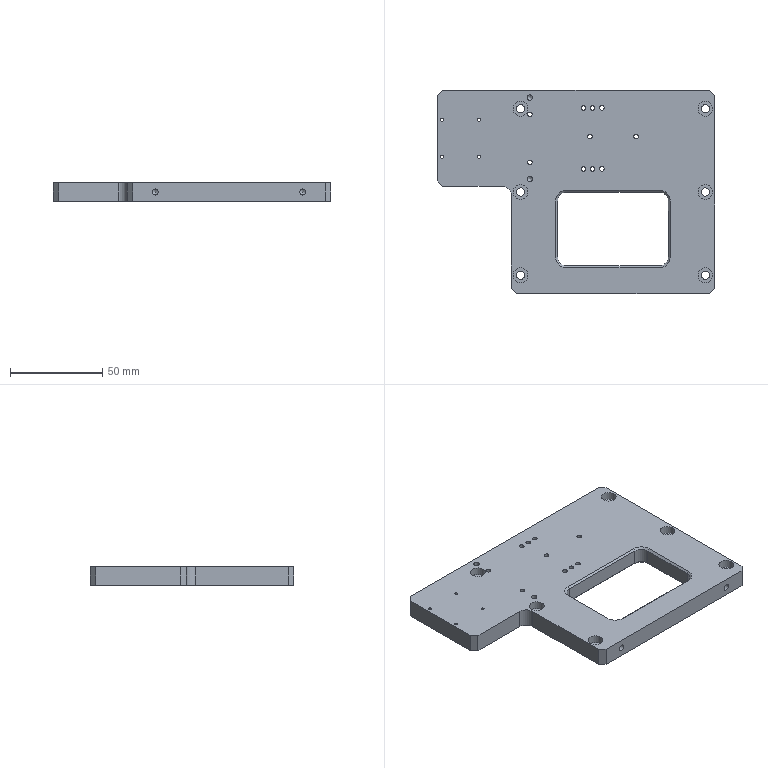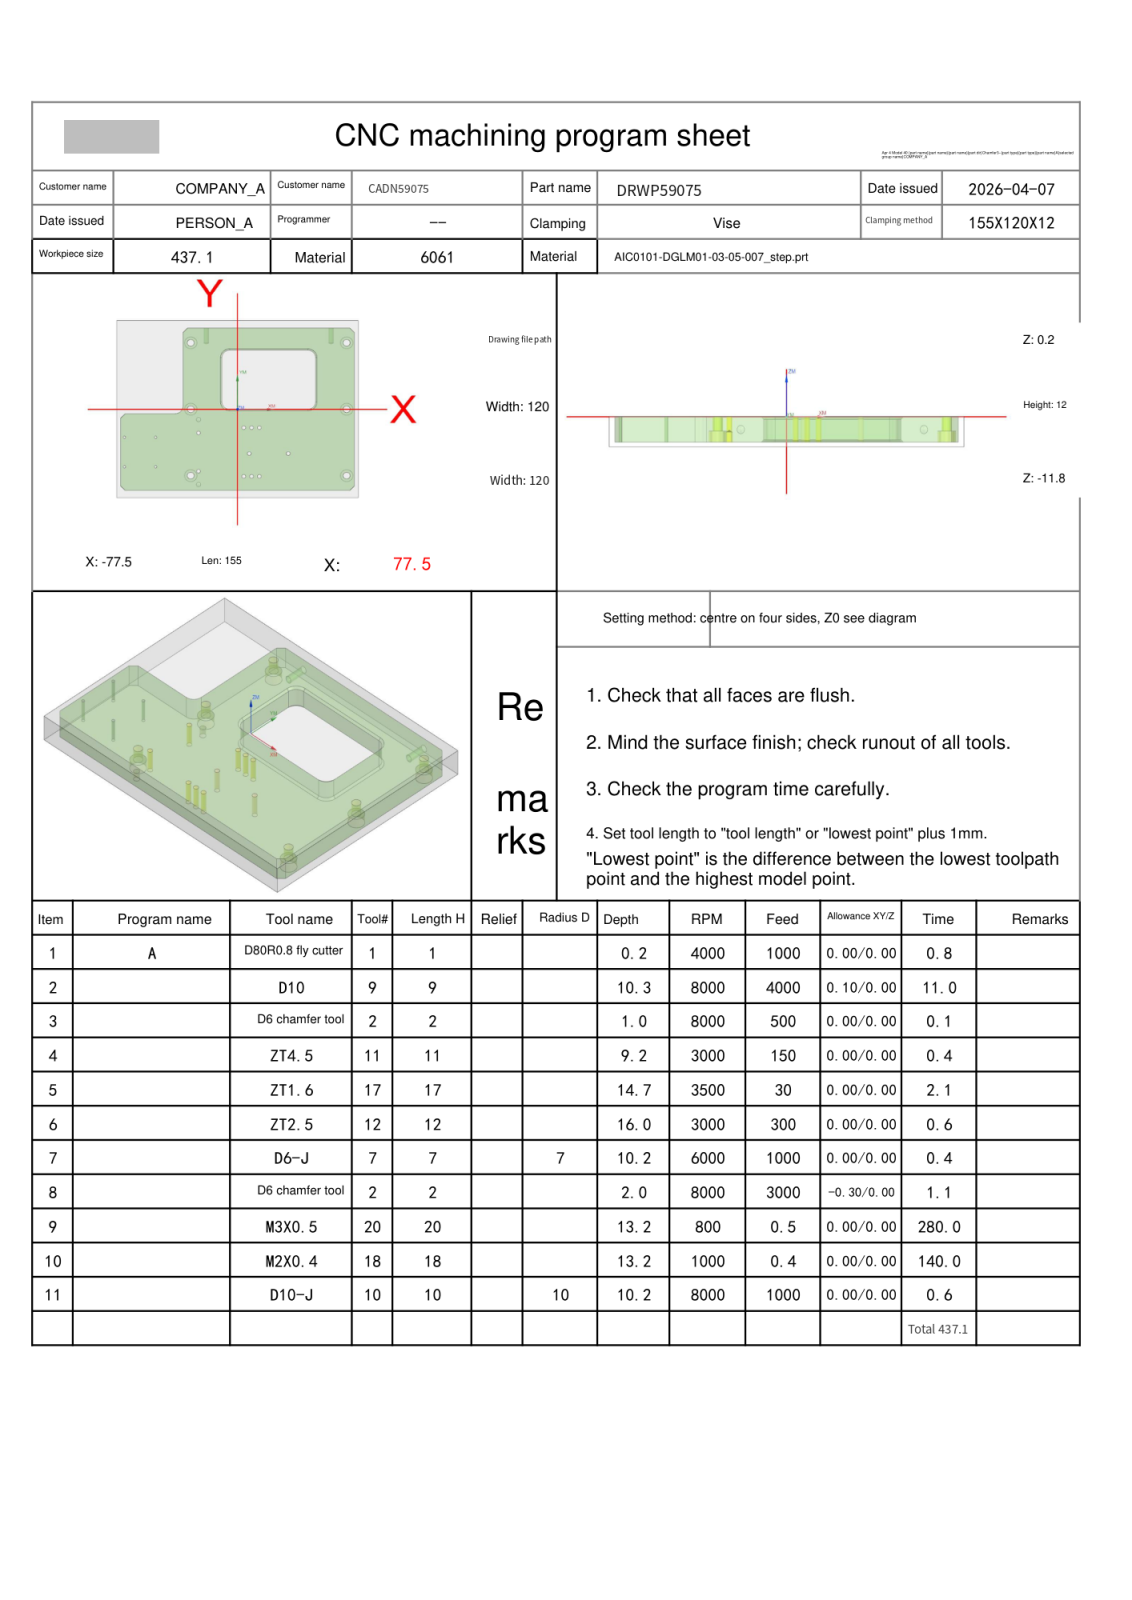NC program | NX | posted by the shop | part box 150 x 110 x 10 mm
Lines 3208 to 3675 of 3675:
N3 T02 M06
(D6 chamfer tool  D=6. R=0. H=02 ce=0.00 di=0.00)
G00 G90 G54 X-30. Y45. M03 S8000
G43 H02 Z20.
M08
G98 G81 X-30. Y45. Z-.8 R1. F500.
Y0.0
X-25. Y-16.
X-52.5 Y-19.
X-72.5
Y-39.
X-52.5
X-30. Y-45.
X-25. Y-42.
X4. Y-45.5
X9.
X14.
X7.5 Y-30.
X4. Y-12.5
X9.
X14.
X32.5 Y-30.
X70. Y-45.
Y0.0
Y45.
G80
G00 Z20.
G91 G28 Z0.0
M05
M09
G91 G28 Z0.0
M01
N4 T11 M06
(ZT4.5 D=4.5 DR_a=118 H=11)
G00 G90 G54 X-30. Y45. M03 S3000
G43 H11 Z20.
M08
G98 G83 X-30. Y45. Z-8.952 R1. F150. Q3.
Y0.0
Y-45.
X70.
Y0.0
Y45.
G80
G00 Z20.
G91 G28 Z0.0
M05
M09
G91 G28 Z0.0
M01
N5 T17 M06
(ZT1.6 D=1.6 DR_a=118 H=17)
G00 G90 G54 X-52.5 Y-39. M03 S3500
G43 H17 Z20.
M08
G98 G83 X-52.5 Y-39. Z-14.481 R1. F30. Q1.
Y-19.
X-72.5
Y-39.
G80
G00 Z20.
G91 G28 Z0.0
M05
M09
G91 G28 Z0.0
M01
N6 T12 M06
(ZT2.5 D=2.5 DR_a=118 H=12)
G00 G90 G54 X32.5 Y-30. M03 S3000
G43 H12 Z20.
M08
G98 G83 X32.5 Y-30. Z-15.751 R1. F300. Q2.
X14. Y-12.5
X9.
X4.
X7.5 Y-30.
X14. Y-45.5
X9.
X4.
X-25. Y-42.
Y-16.
G80
G00 Z20.
G91 G28 Z0.0
M05
M09
G91 G28 Z0.0
M01
N7 T07 M06
(D6-J  D=6. R=0. H=07 ce=0.00 di=0.00)
G00 G90 G54 X46. Y34.8 M03 S6000
G43 H07 Z20.
M08
Z-8.
G01 Z-8.5 F1000.
G41 D07
Y36.
G03 X45. Y37. I-1. J0.0
G01 X-5.
G03 X-7. Y35. I0.0 J-2.
G01 Y5.
G03 X-5. Y3. I2. J0.0
G01 X45.
G03 X47. Y5. I0.0 J2.
G01 Y35.
G03 X45. Y37. I-2. J0.0
G01 X44.5
G03 X43.5 Y36. I0.0 J-1.
G01 G40 Y35.8
Z-8.
G00 Z20.
G00 G90 X46. Y34.9 M03 S6000
Z20.
Z-9.5
G01 Z-10. F1000.
G41 D07
Y36.
G03 X45. Y37. I-1. J0.0
G01 X-5.
G03 X-7. Y35. I0.0 J-2.
G01 Y5.
G03 X-5. Y3. I2. J0.0
G01 X45.
G03 X47. Y5. I0.0 J2.
G01 Y35.
G03 X45. Y37. I-2. J0.0
G01 X44.5
G03 X43.5 Y36. I0.0 J-1.
G01 G40 Y35.9
Z-9.5
G00 Z20.
G91 G28 Z0.0
M05
M09
G91 G28 Z0.0
M01
N8 T02 M06
(D6 chamfer tool  D=6. R=0. H=02 ce=0.00 di=0.00)
G00 G90 G54 X.25 Y-57.128 M03 S8000
G43 H02 Z20.
M08
Z2.099
G01 Z-1.5 F3000.
G03 X.33 Y-56.828 I-.52 J.3
X.03 Y-56.308 I-.6 J0.0
G01 X0.0 Y-56.3
X-72.
X-72.254 Y-56.275
X-72.497 Y-56.201
X-72.722 Y-56.081
X-72.919 Y-55.919
X-75.919 Y-52.919
X-76.081 Y-52.722
X-76.201 Y-52.497
X-76.275 Y-52.254
X-76.3 Y-52.
Y-6.
X-76.275 Y-5.746
X-76.201 Y-5.503
X-76.081 Y-5.278
X-75.919 Y-5.081
X-72.919 Y-2.081
X-72.722 Y-1.919
X-72.497 Y-1.799
X-72.254 Y-1.725
X-72. Y-1.7
X-40.
G03 X-36.3 Y2. I0.0 J3.7
G01 Y52.
X-36.275 Y52.254
X-36.201 Y52.497
X-36.081 Y52.722
X-35.919 Y52.919
X-32.919 Y55.919
X-32.722 Y56.081
X-32.497 Y56.201
X-32.254 Y56.275
X-32. Y56.3
X72.
X72.254 Y56.275
X72.497 Y56.201
X72.722 Y56.081
X72.919 Y55.919
X75.919 Y52.919
X76.081 Y52.722
X76.201 Y52.497
X76.275 Y52.254
X76.3 Y52.
Y-52.
X76.275 Y-52.254
X76.201 Y-52.497
X76.081 Y-52.722
X75.919 Y-52.919
X72.919 Y-55.919
X72.722 Y-56.081
X72.497 Y-56.201
X72.254 Y-56.275
X72. Y-56.3
X0.0
X-.03 Y-56.308
G03 X-.33 Y-56.828 I.3 J-.52
X-.25 Y-57.128 I.6 J0.0
G01 Z2.099
G00 Z20.
G00 G90 X-52.5 Y-39. M03 S8000
Z20.
G98 G81 X-52.5 Y-39. Z-1.2 R3. F500.
Y-19.
X-72.5
Y-39.
G80
G00 Z20.
G00 G90 X32.5 Y-30. M03 S8000
Z20.
G98 G81 X32.5 Y-30. Z-1.75 R3. F500.
X14. Y-12.5
X9.
X4.
X7.5 Y-30.
X14. Y-45.5
X9.
X4.
X-25. Y-42.
Y-16.
G80
G00 Z20.
G00 G90 X69.982 Y45.55 M03 S8000
Z20.
Z-.5
G01 Z-1. F500.
X69.95 Y46.5
G03 X68.45 Y45. I0.0 J-1.5
X70. Y43.45 I1.55 J0.0
X71.55 Y45. I0.0 J1.55
X70. Y46.55 I-1.55 J0.0
X68.45 Y45. I0.0 J-1.55
X69.95 Y43.5 I1.5 J0.0
G01 X69.982 Y44.45
Z-.5
G00 Z20.
Y.55
Z-.5
G01 Z-1.
X69.95 Y1.5
G03 X68.45 Y0.0 I0.0 J-1.5
X70. Y-1.55 I1.55 J0.0
X71.55 Y0.0 I0.0 J1.55
X70. Y1.55 I-1.55 J0.0
X68.45 Y0.0 I0.0 J-1.55
X69.95 Y-1.5 I1.5 J0.0
G01 X69.982 Y-.55
Z-.5
G00 Z20.
Y-44.45
Z-.5
G01 Z-1.
X69.95 Y-43.5
G03 X68.45 Y-45. I0.0 J-1.5
X70. Y-46.55 I1.55 J0.0
X71.55 Y-45. I0.0 J1.55
X70. Y-43.45 I-1.55 J0.0
X68.45 Y-45. I0.0 J-1.55
X69.95 Y-46.5 I1.5 J0.0
G01 X69.982 Y-45.55
Z-.5
G00 Z20.
X-30.018 Y-44.45
Z-.5
G01 Z-1.
X-30.05 Y-43.5
G03 X-31.55 Y-45. I0.0 J-1.5
X-30. Y-46.55 I1.55 J0.0
X-28.45 Y-45. I0.0 J1.55
X-30. Y-43.45 I-1.55 J0.0
X-31.55 Y-45. I0.0 J-1.55
X-30.05 Y-46.5 I1.5 J0.0
G01 X-30.018 Y-45.55
Z-.5
G00 Z20.
Y.55
Z-.5
G01 Z-1.
X-30.05 Y1.5
G03 X-31.55 Y0.0 I0.0 J-1.5
X-30. Y-1.55 I1.55 J0.0
X-28.45 Y0.0 I0.0 J1.55
X-30. Y1.55 I-1.55 J0.0
X-31.55 Y0.0 I0.0 J-1.55
X-30.05 Y-1.5 I1.5 J0.0
G01 X-30.018 Y-.55
Z-.5
G00 Z20.
Y45.55
Z-.5
G01 Z-1.
X-30.05 Y46.5
G03 X-31.55 Y45. I0.0 J-1.5
X-30. Y43.45 I1.55 J0.0
X-28.45 Y45. I0.0 J1.55
X-30. Y46.55 I-1.55 J0.0
X-31.55 Y45. I0.0 J-1.55
X-30.05 Y43.5 I1.5 J0.0
G01 X-30.018 Y44.45
Z-.5
G00 Z20.
G00 G90 X46.2 Y37.193 M03 S6500
Z20.
Z-.2
G01 Z-1.7 F1500.
Y37.5
G03 X45. Y38.7 I-1.2 J0.0
G01 X-5.
G03 X-8.7 Y35. I0.0 J-3.7
G01 Y5.
G03 X-5. Y1.3 I3.7 J0.0
G01 X45.
G03 X48.7 Y5. I0.0 J3.7
G01 Y35.
G03 X48.693 Y35.231 I-3.7 J0.0
G01 X48.681 Y35.372
G03 X48.648 Y35.617 I-3.681 J-.372
X46.911 Y38.169 I-3.648 J-.617
X46.423 Y38.416 I-1.911 J-3.169
X45. Y38.7 I-1.423 J-3.416
G01 X44.6
G03 X43.4 Y37.5 I0.0 J-1.2
G01 X46.2 Y37.7
G03 X45. Y38.9 I-1.2 J0.0
G01 X-5.
G03 X-8.9 Y35. I0.0 J-3.9
G01 Y5.
G03 X-5. Y1.1 I3.9 J0.0
G01 X45.
G03 X48.9 Y5. I0.0 J3.9
G01 Y35.
G03 X48.892 Y35.243 I-3.9 J0.0
G01 X48.88 Y35.392
G03 X48.845 Y35.65 I-3.88 J-.392
X47.014 Y38.34 I-3.845 J-.65
X46.5 Y38.6 I-2.014 J-3.34
X45. Y38.9 I-1.5 J-3.6
G01 X44.6
G03 X43.4 Y37.7 I0.0 J-1.2
G01 X46.2 Y37.9
G03 X45. Y39.1 I-1.2 J0.0
G01 X-5.
G03 X-9.1 Y35. I0.0 J-4.1
G01 Y5.
G03 X-5. Y.9 I4.1 J0.0
G01 X45.
G03 X49.1 Y5. I0.0 J4.1
G01 Y35.
G03 X49.092 Y35.256 I-4.1 J0.0
G01 X49.089 Y35.334
X49.079 Y35.412
G03 X49.043 Y35.684 I-4.079 J-.412
X47.117 Y38.511 I-4.043 J-.684
X46.576 Y38.785 I-2.117 J-3.511
X45. Y39.1 I-1.576 J-3.785
G01 X44.6
G03 X43.4 Y37.9 I0.0 J-1.2
G01 X46.2 Y38.1
G03 X45. Y39.3 I-1.2 J0.0
G01 X-5.
G03 X-9.3 Y35. I0.0 J-4.3
G01 Y5.
G03 X-5. Y.7 I4.3 J0.0
G01 X45.
G03 X49.3 Y5. I0.0 J4.3
G01 Y35.
G03 X49.292 Y35.268 I-4.3 J0.0
G01 X49.289 Y35.351
X49.278 Y35.432
G03 X49.24 Y35.717 I-4.278 J-.432
X45. Y39.3 I-4.24 J-.717
G01 X44.6
G03 X43.4 Y38.1 I0.0 J-1.2
G01 Z-.2
G00 Z20.
G91 G28 Z0.0
M05
M09
G91 G28 Z0.0
M01
N9 T20 M06
(M3X0.5 D=2.5 DR_a=180 H=20)
G00 G90 G54 X32.5 Y-30. M03 S800
G43 H20 Z20.
M08
G95
G98 G84 X32.5 Y-30. Z-13. R1. F.5 Q5.
X14. Y-12.5
X9.
X4.
X7.5 Y-30.
X14. Y-45.5
X9.
X4.
X-25. Y-42.
Y-16.
G80
G94
G00 Z20.
G91 G28 Z0.0
M05
M09
G91 G28 Z0.0
M01
N10 T18 M06
(M2X0.4 D=1.6 DR_a=180 H=18)
G00 G90 G54 X-52.5 Y-39. M03 S1000
G43 H18 Z20.
M08
G95
G98 G84 X-52.5 Y-39. Z-13. R1. F.4 Q4.
Y-19.
X-72.5
Y-39.
G80
G94
G00 Z20.
G91 G28 Z0.0
M05
M09
G91 G28 Z0.0
M01
N11 T10 M06
(D10-J  D=10. R=0. H=10 ce=0.00 di=0.00)
G00 G90 G54 X73.013 Y-61.116 M03 S8000
G43 H10 Z20.
M08
Z-9.5
G01 Z-10. F1000.
G41 D10
X72.997 Y-60.917
G03 X72. Y-60. I-.997 J-.083
G01 X-72.
G02 X-75.536 Y-58.536 I0.0 J5.
G01 X-78.536 Y-55.536
G02 X-80. Y-52. I3.536 J3.536
G01 Y-6.
G02 X-78.536 Y-2.464 I5. J0.0
G01 X-75.536 Y.536
G02 X-72. Y2. I3.536 J-3.536
G01 X-40.
Y52.
G02 X-38.536 Y55.536 I5. J0.0
G01 X-35.536 Y58.536
G02 X-32. Y60. I3.536 J-3.536
G01 X72.
G02 X75.536 Y58.536 I0.0 J-5.
G01 X78.536 Y55.536
G02 X80. Y52. I-3.536 J-3.536
G01 Y-52.
G02 X78.536 Y-55.536 I-5. J0.0
G01 X75.536 Y-58.536
G02 X72. Y-60. I-3.536 J3.536
G01 X71.5
G03 X70.5 Y-61. I0.0 J-1.
G01 G40 Y-61.2
Z-9.5
G00 Z20.
M05
M09
G91 G28 Z0.0
G91 G28 Y0.0
M30
%